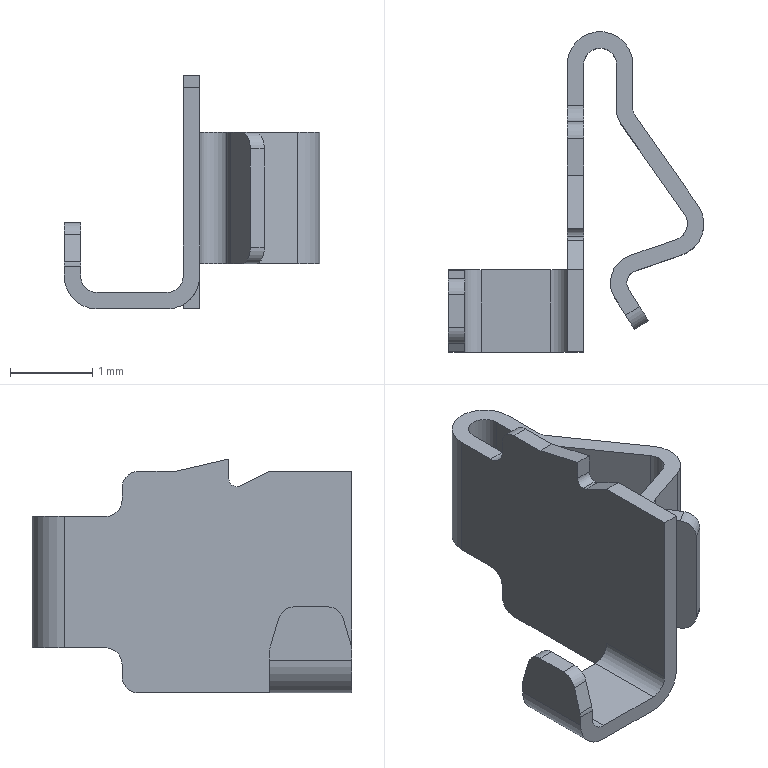Part | Creo | 1 solid | 56 faces | box 3.115 x 3.9 x 2.85 mm | volume 3.729 mm3 | plane 31 | cylinder 25 | commonest cylinder face diameters 0.4 x14 0.8 x4 0.2 x3 0.7 x2 0.3 x1 0.6 x1